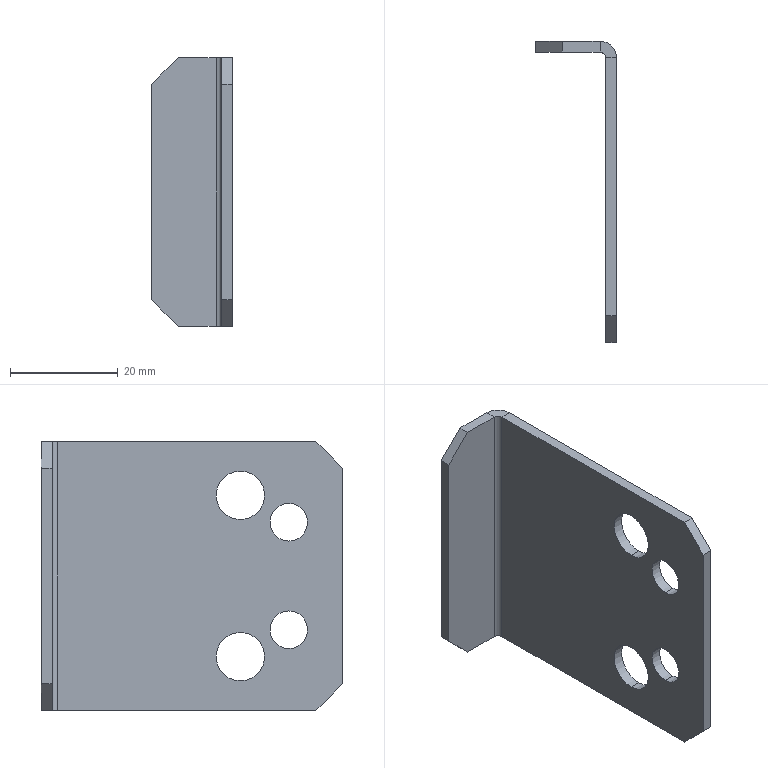Part | STEP file | Electromagnetic lock bracket A | 1 solid | 26 faces | box 15 x 56 x 50 mm | volume 6308 mm3 | plane 16 | cylinder 10 | commonest cylinder face diameters 7 x4 9 x4 2 x1 6 x1